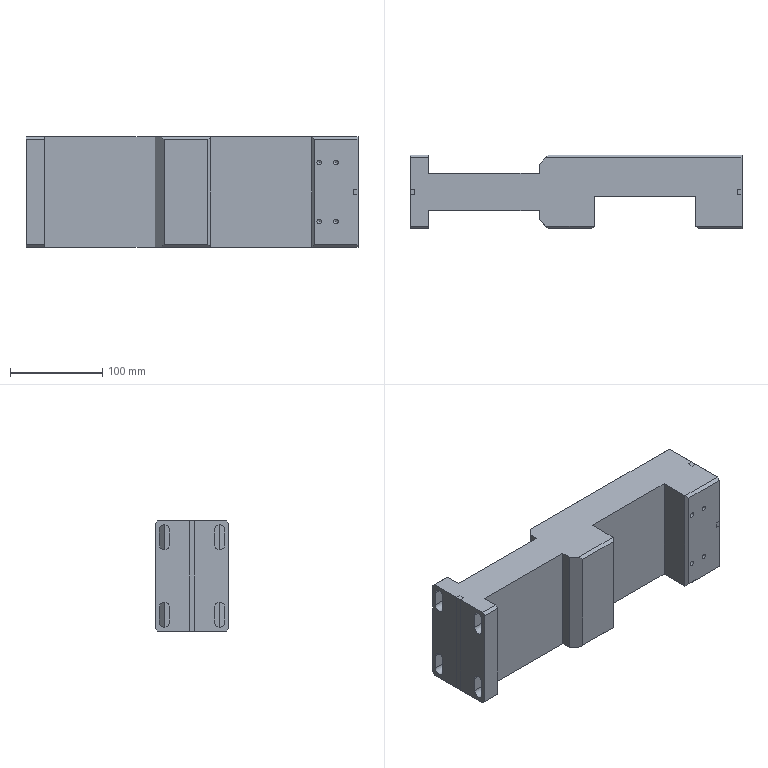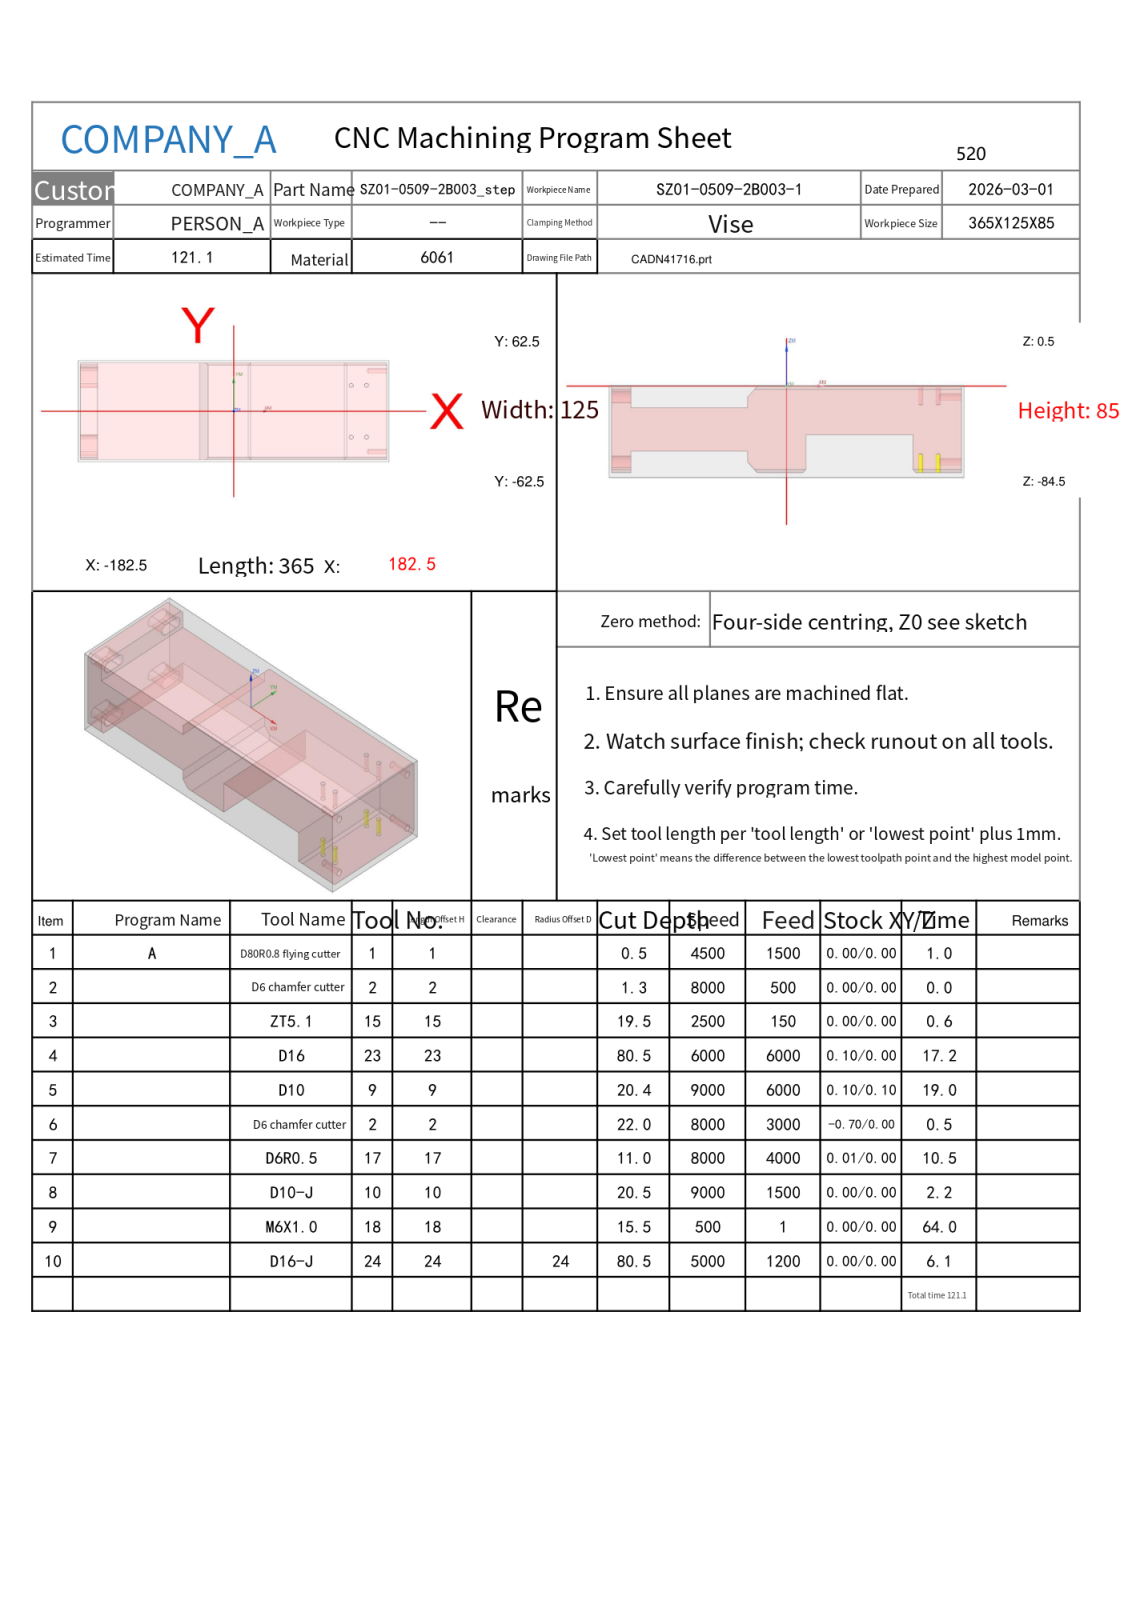NC program | NX | posted by the shop | part box 360 x 80 x 120 mm
Lines 1 to 903 of 6444:
%
O0001
(Machine time: 182.87 MIN)
(===Total Tool:9===)
(T1=D80R0.8 flying cutter D=80.  R=0.8  D-  H01 Z=0.    )
(T2=D6 chamfer cutter   D=6.   R=0.   D-  H02 Z=-21.5 )
(T15=ZT5.1  D=5.1  DR_a=118 D-  H15 Z=-19.  )
(T23=D16    D=16.  R=0.   D-  H23 Z=-80.  )
(T9=D10     D=10.  R=0.   D-  H09 Z=-19.9 )
(T17=D6R0.5 D=6.   R=0.5  D-  H17 Z=-10.5 )
(T10=D10-J  D=10.  R=0.   D10 H10 Z=-20.  )
(T18=M6X1.0 D=5.   DR_a=180 D-  H18 Z=-15.  )
(T24=D16-J  D=16.  R=0.   D24 H24 Z=-80.  )
G80 G90 G17 G49 G40
G91 G28 Z0
M01
N1 T01 M06
(D80R0.8 flying cutter  D=80. R=0.8 H=01 ce=0.00 di=0.00)
G00 G90 G54 X225. Y-50. M03 S4500
G43 H01 Z50.
M08
Z2.
G01 Z0.0 F1500.
X220.
X-220.
Y0.0
X220.
Y50.
X-220.
X-225.
Z2.
G00 Z50.
G91 G28 Z0.0
M05
M09
G91 G28 Z0.0
M01
N2 T02 M06
(D6 chamfer cutter  D=6. R=0. H=02 ce=0.00 di=0.00)
G00 G90 G54 X138. Y-32. M03 S8000
G43 H02 Z50.
M08
G98 G81 X138. Y-32. Z-.8 R1. F500.
X156.
Y32.
X138.
G80
G00 Z50.
G91 G28 Z0.0
M05
M09
G91 G28 Z0.0
M01
N3 T15 M06
(ZT5.1 D=5.1 DR_a=118 H=15)
G00 G90 G54 X138. Y-32. M03 S2500
G43 H15 Z50.
M08
G98 G83 X138. Y-32. Z-19. R1. F150. Q3.
X156.
Y32.
X138.
G80
G00 Z50.
G91 G28 Z0.0
M05
M09
G91 G28 Z0.0
M01
N4 T23 M06
(D16  D=16. R=0. H=23 ce=0.10 di=0.00)
G00 G90 G54 X0.0 Y68.1 M03 S6000
G43 H23 Z50.
M08
Z.5
G01 X180. Z.358 F6000.
G02 X188.1 Y60. Z.348 I0.0 J-8.1
G01 Y-60. Z.253
G02 X180. Y-68.1 Z.243 I-8.1 J0.0
G01 X-180. Z-.04
G02 X-188.1 Y-60. Z-.05 I0.0 J8.1
G01 Y60. Z-.145
G02 X-180. Y68.1 Z-.155 I8.1 J0.0
G01 X180. Z-.439
G02 X188.1 Y60. Z-.449 I0.0 J-8.1
G01 Y-60. Z-.544
G02 X180. Y-68.1 Z-.554 I-8.1 J0.0
G01 X-180. Z-.837
G02 X-188.1 Y-60. Z-.847 I0.0 J8.1
G01 Y60. Z-.942
G02 X-180. Y68.1 Z-.952 I8.1 J0.0
G01 X180. Z-1.236
G02 X188.1 Y60. Z-1.246 I0.0 J-8.1
G01 Y-60. Z-1.341
G02 X180. Y-68.1 Z-1.351 I-8.1 J0.0
G01 X-180. Z-1.634
G02 X-188.1 Y-60. Z-1.645 I0.0 J8.1
G01 Y60. Z-1.739
G02 X-180. Y68.1 Z-1.749 I8.1 J0.0
G01 X180. Z-2.033
G02 X188.1 Y60. Z-2.043 I0.0 J-8.1
G01 Y-60. Z-2.138
G02 X180. Y-68.1 Z-2.148 I-8.1 J0.0
G01 X-180. Z-2.432
G02 X-188.1 Y-60. Z-2.442 I0.0 J8.1
G01 Y60. Z-2.536
G02 X-180. Y68.1 Z-2.546 I8.1 J0.0
G01 X180. Z-2.83
G02 X188.1 Y60. Z-2.84 I0.0 J-8.1
G01 Y-60. Z-2.935
G02 X180. Y-68.1 Z-2.945 I-8.1 J0.0
G01 X-180. Z-3.229
G02 X-188.1 Y-60. Z-3.239 I0.0 J8.1
G01 Y60. Z-3.333
G02 X-180. Y68.1 Z-3.343 I8.1 J0.0
G01 X180. Z-3.627
G02 X188.1 Y60. Z-3.637 I0.0 J-8.1
G01 Y-60. Z-3.732
G02 X180. Y-68.1 Z-3.742 I-8.1 J0.0
G01 X-180. Z-4.026
G02 X-188.1 Y-60. Z-4.036 I0.0 J8.1
G01 Y60. Z-4.13
G02 X-180. Y68.1 Z-4.14 I8.1 J0.0
G01 X180. Z-4.424
G02 X188.1 Y60. Z-4.434 I0.0 J-8.1
G01 Y-60. Z-4.529
G02 X180. Y-68.1 Z-4.539 I-8.1 J0.0
G01 X-180. Z-4.823
G02 X-188.1 Y-60. Z-4.833 I0.0 J8.1
G01 Y60. Z-4.927
G02 X-180. Y68.1 Z-4.937 I8.1 J0.0
G01 X180. Z-5.221
G02 X188.1 Y60. Z-5.231 I0.0 J-8.1
G01 Y-60. Z-5.326
G02 X180. Y-68.1 Z-5.336 I-8.1 J0.0
G01 X-180. Z-5.62
G02 X-188.1 Y-60. Z-5.63 I0.0 J8.1
G01 Y60. Z-5.724
G02 X-180. Y68.1 Z-5.734 I8.1 J0.0
G01 X180. Z-6.018
G02 X188.1 Y60. Z-6.028 I0.0 J-8.1
G01 Y-60. Z-6.123
G02 X180. Y-68.1 Z-6.133 I-8.1 J0.0
G01 X-180. Z-6.417
G02 X-188.1 Y-60. Z-6.427 I0.0 J8.1
G01 Y60. Z-6.521
G02 X-180. Y68.1 Z-6.531 I8.1 J0.0
G01 X180. Z-6.815
G02 X188.1 Y60. Z-6.825 I0.0 J-8.1
G01 Y-60. Z-6.92
G02 X180. Y-68.1 Z-6.93 I-8.1 J0.0
G01 X-180. Z-7.214
G02 X-188.1 Y-60. Z-7.224 I0.0 J8.1
G01 Y60. Z-7.318
G02 X-180. Y68.1 Z-7.328 I8.1 J0.0
G01 X180. Z-7.612
G02 X188.1 Y60. Z-7.622 I0.0 J-8.1
G01 Y-60. Z-7.717
G02 X180. Y-68.1 Z-7.727 I-8.1 J0.0
G01 X-180. Z-8.011
G02 X-188.1 Y-60. Z-8.021 I0.0 J8.1
G01 Y60. Z-8.115
G02 X-180. Y68.1 Z-8.125 I8.1 J0.0
G01 X180. Z-8.409
G02 X188.1 Y60. Z-8.419 I0.0 J-8.1
G01 Y-60. Z-8.514
G02 X180. Y-68.1 Z-8.524 I-8.1 J0.0
G01 X-180. Z-8.808
G02 X-188.1 Y-60. Z-8.818 I0.0 J8.1
G01 Y60. Z-8.912
G02 X-180. Y68.1 Z-8.922 I8.1 J0.0
G01 X180. Z-9.206
G02 X188.1 Y60. Z-9.216 I0.0 J-8.1
G01 Y-60. Z-9.311
G02 X180. Y-68.1 Z-9.321 I-8.1 J0.0
G01 X-180. Z-9.605
G02 X-188.1 Y-60. Z-9.615 I0.0 J8.1
G01 Y60. Z-9.709
G02 X-180. Y68.1 Z-9.719 I8.1 J0.0
G01 X180. Z-10.003
G02 X188.1 Y60. Z-10.013 I0.0 J-8.1
G01 Y-60. Z-10.108
G02 X180. Y-68.1 Z-10.118 I-8.1 J0.0
G01 X-180. Z-10.402
G02 X-188.1 Y-60. Z-10.412 I0.0 J8.1
G01 Y60. Z-10.506
G02 X-180. Y68.1 Z-10.516 I8.1 J0.0
G01 X180. Z-10.8
G02 X188.1 Y60. Z-10.81 I0.0 J-8.1
G01 Y-60. Z-10.905
G02 X180. Y-68.1 Z-10.915 I-8.1 J0.0
G01 X-180. Z-11.199
G02 X-188.1 Y-60. Z-11.209 I0.0 J8.1
G01 Y60. Z-11.303
G02 X-180. Y68.1 Z-11.314 I8.1 J0.0
G01 X180. Z-11.597
G02 X188.1 Y60. Z-11.607 I0.0 J-8.1
G01 Y-60. Z-11.702
G02 X180. Y-68.1 Z-11.712 I-8.1 J0.0
G01 X-180. Z-11.996
G02 X-188.1 Y-60. Z-12.006 I0.0 J8.1
G01 Y60. Z-12.101
G02 X-180. Y68.1 Z-12.111 I8.1 J0.0
G01 X180. Z-12.394
G02 X188.1 Y60. Z-12.404 I0.0 J-8.1
G01 Y-60. Z-12.499
G02 X180. Y-68.1 Z-12.509 I-8.1 J0.0
G01 X-180. Z-12.793
G02 X-188.1 Y-60. Z-12.803 I0.0 J8.1
G01 Y60. Z-12.898
G02 X-180. Y68.1 Z-12.908 I8.1 J0.0
G01 X180. Z-13.191
G02 X188.1 Y60. Z-13.201 I0.0 J-8.1
G01 Y-60. Z-13.296
G02 X180. Y-68.1 Z-13.306 I-8.1 J0.0
G01 X-180. Z-13.59
G02 X-188.1 Y-60. Z-13.6 I0.0 J8.1
G01 Y60. Z-13.695
G02 X-180. Y68.1 Z-13.705 I8.1 J0.0
G01 X180. Z-13.988
G02 X188.1 Y60. Z-13.998 I0.0 J-8.1
G01 Y-60. Z-14.093
G02 X180. Y-68.1 Z-14.103 I-8.1 J0.0
G01 X-180. Z-14.387
G02 X-188.1 Y-60. Z-14.397 I0.0 J8.1
G01 Y60. Z-14.492
G02 X-180. Y68.1 Z-14.502 I8.1 J0.0
G01 X180. Z-14.785
G02 X188.1 Y60. Z-14.796 I0.0 J-8.1
G01 Y-60. Z-14.89
G02 X180. Y-68.1 Z-14.9 I-8.1 J0.0
G01 X-180. Z-15.184
G02 X-188.1 Y-60. Z-15.194 I0.0 J8.1
G01 Y60. Z-15.289
G02 X-180. Y68.1 Z-15.299 I8.1 J0.0
G01 X180. Z-15.583
G02 X188.1 Y60. Z-15.593 I0.0 J-8.1
G01 Y-60. Z-15.687
G02 X180. Y-68.1 Z-15.697 I-8.1 J0.0
G01 X-180. Z-15.981
G02 X-188.1 Y-60. Z-15.991 I0.0 J8.1
G01 Y60. Z-16.086
G02 X-180. Y68.1 Z-16.096 I8.1 J0.0
G01 X180. Z-16.38
G02 X188.1 Y60. Z-16.39 I0.0 J-8.1
G01 Y-60. Z-16.484
G02 X180. Y-68.1 Z-16.494 I-8.1 J0.0
G01 X-180. Z-16.778
G02 X-188.1 Y-60. Z-16.788 I0.0 J8.1
G01 Y60. Z-16.883
G02 X-180. Y68.1 Z-16.893 I8.1 J0.0
G01 X180. Z-17.177
G02 X188.1 Y60. Z-17.187 I0.0 J-8.1
G01 Y-60. Z-17.281
G02 X180. Y-68.1 Z-17.291 I-8.1 J0.0
G01 X-180. Z-17.575
G02 X-188.1 Y-60. Z-17.585 I0.0 J8.1
G01 Y60. Z-17.68
G02 X-180. Y68.1 Z-17.69 I8.1 J0.0
G01 X180. Z-17.974
G02 X188.1 Y60. Z-17.984 I0.0 J-8.1
G01 Y-60. Z-18.078
G02 X180. Y-68.1 Z-18.088 I-8.1 J0.0
G01 X-180. Z-18.372
G02 X-188.1 Y-60. Z-18.382 I0.0 J8.1
G01 Y60. Z-18.477
G02 X-180. Y68.1 Z-18.487 I8.1 J0.0
G01 X180. Z-18.771
G02 X188.1 Y60. Z-18.781 I0.0 J-8.1
G01 Y-60. Z-18.875
G02 X180. Y-68.1 Z-18.885 I-8.1 J0.0
G01 X-180. Z-19.169
G02 X-188.1 Y-60. Z-19.179 I0.0 J8.1
G01 Y60. Z-19.274
G02 X-180. Y68.1 Z-19.284 I8.1 J0.0
G01 X180. Z-19.568
G02 X188.1 Y60. Z-19.578 I0.0 J-8.1
G01 Y-60. Z-19.672
G02 X180. Y-68.1 Z-19.682 I-8.1 J0.0
G01 X-180. Z-19.966
G02 X-188.1 Y-60. Z-19.976 I0.0 J8.1
G01 Y60. Z-20.071
G02 X-180. Y68.1 Z-20.081 I8.1 J0.0
G01 X180. Z-20.365
G02 X188.1 Y60. Z-20.375 I0.0 J-8.1
G01 Y-60. Z-20.469
G02 X180. Y-68.1 Z-20.479 I-8.1 J0.0
G01 X-180. Z-20.763
G02 X-188.1 Y-60. Z-20.773 I0.0 J8.1
G01 Y60. Z-20.868
G02 X-180. Y68.1 Z-20.878 I8.1 J0.0
G01 X180. Z-21.162
G02 X188.1 Y60. Z-21.172 I0.0 J-8.1
G01 Y-60. Z-21.266
G02 X180. Y-68.1 Z-21.276 I-8.1 J0.0
G01 X-180. Z-21.56
G02 X-188.1 Y-60. Z-21.57 I0.0 J8.1
G01 Y60. Z-21.665
G02 X-180. Y68.1 Z-21.675 I8.1 J0.0
G01 X180. Z-21.959
G02 X188.1 Y60. Z-21.969 I0.0 J-8.1
G01 Y-60. Z-22.063
G02 X180. Y-68.1 Z-22.073 I-8.1 J0.0
G01 X-180. Z-22.357
G02 X-188.1 Y-60. Z-22.367 I0.0 J8.1
G01 Y60. Z-22.462
G02 X-180. Y68.1 Z-22.472 I8.1 J0.0
G01 X180. Z-22.756
G02 X188.1 Y60. Z-22.766 I0.0 J-8.1
G01 Y-60. Z-22.86
G02 X180. Y-68.1 Z-22.87 I-8.1 J0.0
G01 X-180. Z-23.154
G02 X-188.1 Y-60. Z-23.164 I0.0 J8.1
G01 Y60. Z-23.259
G02 X-180. Y68.1 Z-23.269 I8.1 J0.0
G01 X180. Z-23.553
G02 X188.1 Y60. Z-23.563 I0.0 J-8.1
G01 Y-60. Z-23.657
G02 X180. Y-68.1 Z-23.667 I-8.1 J0.0
G01 X-180. Z-23.951
G02 X-188.1 Y-60. Z-23.961 I0.0 J8.1
G01 Y60. Z-24.056
G02 X-180. Y68.1 Z-24.066 I8.1 J0.0
G01 X180. Z-24.35
G02 X188.1 Y60. Z-24.36 I0.0 J-8.1
G01 Y-60. Z-24.454
G02 X180. Y-68.1 Z-24.465 I-8.1 J0.0
G01 X-180. Z-24.748
G02 X-188.1 Y-60. Z-24.758 I0.0 J8.1
G01 Y60. Z-24.853
G02 X-180. Y68.1 Z-24.863 I8.1 J0.0
G01 X180. Z-25.147
G02 X188.1 Y60. Z-25.157 I0.0 J-8.1
G01 Y-60. Z-25.252
G02 X180. Y-68.1 Z-25.262 I-8.1 J0.0
G01 X-180. Z-25.545
G02 X-188.1 Y-60. Z-25.555 I0.0 J8.1
G01 Y60. Z-25.65
G02 X-180. Y68.1 Z-25.66 I8.1 J0.0
G01 X180. Z-25.944
G02 X188.1 Y60. Z-25.954 I0.0 J-8.1
G01 Y-60. Z-26.049
G02 X180. Y-68.1 Z-26.059 I-8.1 J0.0
G01 X-180. Z-26.342
G02 X-188.1 Y-60. Z-26.352 I0.0 J8.1
G01 Y60. Z-26.447
G02 X-180. Y68.1 Z-26.457 I8.1 J0.0
G01 X180. Z-26.741
G02 X188.1 Y60. Z-26.751 I0.0 J-8.1
G01 Y-60. Z-26.846
G02 X180. Y-68.1 Z-26.856 I-8.1 J0.0
G01 X-180. Z-27.139
G02 X-188.1 Y-60. Z-27.149 I0.0 J8.1
G01 Y60. Z-27.244
G02 X-180. Y68.1 Z-27.254 I8.1 J0.0
G01 X180. Z-27.538
G02 X188.1 Y60. Z-27.548 I0.0 J-8.1
G01 Y-60. Z-27.643
G02 X180. Y-68.1 Z-27.653 I-8.1 J0.0
G01 X-180. Z-27.936
G02 X-188.1 Y-60. Z-27.947 I0.0 J8.1
G01 Y60. Z-28.041
G02 X-180. Y68.1 Z-28.051 I8.1 J0.0
G01 X180. Z-28.335
G02 X188.1 Y60. Z-28.345 I0.0 J-8.1
G01 Y-60. Z-28.44
G02 X180. Y-68.1 Z-28.45 I-8.1 J0.0
G01 X-180. Z-28.734
G02 X-188.1 Y-60. Z-28.744 I0.0 J8.1
G01 Y60. Z-28.838
G02 X-180. Y68.1 Z-28.848 I8.1 J0.0
G01 X180. Z-29.132
G02 X188.1 Y60. Z-29.142 I0.0 J-8.1
G01 Y-60. Z-29.237
G02 X180. Y-68.1 Z-29.247 I-8.1 J0.0
G01 X-180. Z-29.531
G02 X-188.1 Y-60. Z-29.541 I0.0 J8.1
G01 Y60. Z-29.635
G02 X-180. Y68.1 Z-29.645 I8.1 J0.0
G01 X180. Z-29.929
G02 X188.1 Y60. Z-29.939 I0.0 J-8.1
G01 Y-60. Z-30.034
G02 X180. Y-68.1 Z-30.044 I-8.1 J0.0
G01 X-180. Z-30.328
G02 X-188.1 Y-60. Z-30.338 I0.0 J8.1
G01 Y60. Z-30.432
G02 X-180. Y68.1 Z-30.442 I8.1 J0.0
G01 X180. Z-30.726
G02 X188.1 Y60. Z-30.736 I0.0 J-8.1
G01 Y-60. Z-30.831
G02 X180. Y-68.1 Z-30.841 I-8.1 J0.0
G01 X-180. Z-31.125
G02 X-188.1 Y-60. Z-31.135 I0.0 J8.1
G01 Y60. Z-31.229
G02 X-180. Y68.1 Z-31.239 I8.1 J0.0
G01 X180. Z-31.523
G02 X188.1 Y60. Z-31.533 I0.0 J-8.1
G01 Y-60. Z-31.628
G02 X180. Y-68.1 Z-31.638 I-8.1 J0.0
G01 X-180. Z-31.922
G02 X-188.1 Y-60. Z-31.932 I0.0 J8.1
G01 Y60. Z-32.026
G02 X-180. Y68.1 Z-32.036 I8.1 J0.0
G01 X180. Z-32.32
G02 X188.1 Y60. Z-32.33 I0.0 J-8.1
G01 Y-60. Z-32.425
G02 X180. Y-68.1 Z-32.435 I-8.1 J0.0
G01 X-180. Z-32.719
G02 X-188.1 Y-60. Z-32.729 I0.0 J8.1
G01 Y60. Z-32.823
G02 X-180. Y68.1 Z-32.833 I8.1 J0.0
G01 X180. Z-33.117
G02 X188.1 Y60. Z-33.127 I0.0 J-8.1
G01 Y-60. Z-33.222
G02 X180. Y-68.1 Z-33.232 I-8.1 J0.0
G01 X-180. Z-33.516
G02 X-188.1 Y-60. Z-33.526 I0.0 J8.1
G01 Y60. Z-33.62
G02 X-180. Y68.1 Z-33.63 I8.1 J0.0
G01 X180. Z-33.914
G02 X188.1 Y60. Z-33.924 I0.0 J-8.1
G01 Y-60. Z-34.019
G02 X180. Y-68.1 Z-34.029 I-8.1 J0.0
G01 X-180. Z-34.313
G02 X-188.1 Y-60. Z-34.323 I0.0 J8.1
G01 Y60. Z-34.417
G02 X-180. Y68.1 Z-34.427 I8.1 J0.0
G01 X180. Z-34.711
G02 X188.1 Y60. Z-34.721 I0.0 J-8.1
G01 Y-60. Z-34.816
G02 X180. Y-68.1 Z-34.826 I-8.1 J0.0
G01 X-180. Z-35.11
G02 X-188.1 Y-60. Z-35.12 I0.0 J8.1
G01 Y60. Z-35.214
G02 X-180. Y68.1 Z-35.224 I8.1 J0.0
G01 X180. Z-35.508
G02 X188.1 Y60. Z-35.518 I0.0 J-8.1
G01 Y-60. Z-35.613
G02 X180. Y-68.1 Z-35.623 I-8.1 J0.0
G01 X-180. Z-35.907
G02 X-188.1 Y-60. Z-35.917 I0.0 J8.1
G01 Y60. Z-36.011
G02 X-180. Y68.1 Z-36.021 I8.1 J0.0
G01 X180. Z-36.305
G02 X188.1 Y60. Z-36.315 I0.0 J-8.1
G01 Y-60. Z-36.41
G02 X180. Y-68.1 Z-36.42 I-8.1 J0.0
G01 X-180. Z-36.704
G02 X-188.1 Y-60. Z-36.714 I0.0 J8.1
G01 Y60. Z-36.808
G02 X-180. Y68.1 Z-36.818 I8.1 J0.0
G01 X180. Z-37.102
G02 X188.1 Y60. Z-37.112 I0.0 J-8.1
G01 Y-60. Z-37.207
G02 X180. Y-68.1 Z-37.217 I-8.1 J0.0
G01 X-180. Z-37.501
G02 X-188.1 Y-60. Z-37.511 I0.0 J8.1
G01 Y60. Z-37.605
G02 X-180. Y68.1 Z-37.616 I8.1 J0.0
G01 X180. Z-37.899
G02 X188.1 Y60. Z-37.909 I0.0 J-8.1
G01 Y-60. Z-38.004
G02 X180. Y-68.1 Z-38.014 I-8.1 J0.0
G01 X-180. Z-38.298
G02 X-188.1 Y-60. Z-38.308 I0.0 J8.1
G01 Y60. Z-38.403
G02 X-180. Y68.1 Z-38.413 I8.1 J0.0
G01 X180. Z-38.696
G02 X188.1 Y60. Z-38.706 I0.0 J-8.1
G01 Y-60. Z-38.801
G02 X180. Y-68.1 Z-38.811 I-8.1 J0.0
G01 X-180. Z-39.095
G02 X-188.1 Y-60. Z-39.105 I0.0 J8.1
G01 Y60. Z-39.2
G02 X-180. Y68.1 Z-39.21 I8.1 J0.0
G01 X180. Z-39.493
G02 X188.1 Y60. Z-39.503 I0.0 J-8.1
G01 Y-60. Z-39.598
G02 X180. Y-68.1 Z-39.608 I-8.1 J0.0
G01 X-180. Z-39.892
G02 X-188.1 Y-60. Z-39.902 I0.0 J8.1
G01 Y60. Z-39.997
G02 X-180. Y68.1 Z-40.007 I8.1 J0.0
G01 X180. Z-40.29
G02 X188.1 Y60. Z-40.3 I0.0 J-8.1
G01 Y-60. Z-40.395
G02 X180. Y-68.1 Z-40.405 I-8.1 J0.0
G01 X-180. Z-40.689
G02 X-188.1 Y-60. Z-40.699 I0.0 J8.1
G01 Y60. Z-40.794
G02 X-180. Y68.1 Z-40.804 I8.1 J0.0
G01 X180. Z-41.087
G02 X188.1 Y60. Z-41.097 I0.0 J-8.1
G01 Y-60. Z-41.192
G02 X180. Y-68.1 Z-41.202 I-8.1 J0.0
G01 X-180. Z-41.486
G02 X-188.1 Y-60. Z-41.496 I0.0 J8.1
G01 Y60. Z-41.591
G02 X-180. Y68.1 Z-41.601 I8.1 J0.0
G01 X180. Z-41.884
G02 X188.1 Y60. Z-41.895 I0.0 J-8.1
G01 Y-60. Z-41.989
G02 X180. Y-68.1 Z-41.999 I-8.1 J0.0
G01 X-180. Z-42.283
G02 X-188.1 Y-60. Z-42.293 I0.0 J8.1
G01 Y60. Z-42.388
G02 X-180. Y68.1 Z-42.398 I8.1 J0.0
G01 X180. Z-42.682
G02 X188.1 Y60. Z-42.692 I0.0 J-8.1
G01 Y-60. Z-42.786
G02 X180. Y-68.1 Z-42.796 I-8.1 J0.0
G01 X-180. Z-43.08
G02 X-188.1 Y-60. Z-43.09 I0.0 J8.1
G01 Y60. Z-43.185
G02 X-180. Y68.1 Z-43.195 I8.1 J0.0
G01 X180. Z-43.479
G02 X188.1 Y60. Z-43.489 I0.0 J-8.1
G01 Y-60. Z-43.583
G02 X180. Y-68.1 Z-43.593 I-8.1 J0.0
G01 X-180. Z-43.877
G02 X-188.1 Y-60. Z-43.887 I0.0 J8.1
G01 Y60. Z-43.982
G02 X-180. Y68.1 Z-43.992 I8.1 J0.0
G01 X180. Z-44.276
G02 X188.1 Y60. Z-44.286 I0.0 J-8.1
G01 Y-60. Z-44.38
G02 X180. Y-68.1 Z-44.39 I-8.1 J0.0
G01 X-180. Z-44.674
G02 X-188.1 Y-60. Z-44.684 I0.0 J8.1
G01 Y60. Z-44.779
G02 X-180. Y68.1 Z-44.789 I8.1 J0.0
G01 X180. Z-45.073
G02 X188.1 Y60. Z-45.083 I0.0 J-8.1
G01 Y-60. Z-45.177
G02 X180. Y-68.1 Z-45.187 I-8.1 J0.0
G01 X-180. Z-45.471
G02 X-188.1 Y-60. Z-45.481 I0.0 J8.1
G01 Y60. Z-45.576
G02 X-180. Y68.1 Z-45.586 I8.1 J0.0
G01 X180. Z-45.87
G02 X188.1 Y60. Z-45.88 I0.0 J-8.1
G01 Y-60. Z-45.974
G02 X180. Y-68.1 Z-45.984 I-8.1 J0.0
G01 X-180. Z-46.268
G02 X-188.1 Y-60. Z-46.278 I0.0 J8.1
G01 Y60. Z-46.373
G02 X-180. Y68.1 Z-46.383 I8.1 J0.0
G01 X180. Z-46.667
G02 X188.1 Y60. Z-46.677 I0.0 J-8.1
G01 Y-60. Z-46.771
G02 X180. Y-68.1 Z-46.781 I-8.1 J0.0
G01 X-180. Z-47.065
G02 X-188.1 Y-60. Z-47.075 I0.0 J8.1
G01 Y60. Z-47.17
G02 X-180. Y68.1 Z-47.18 I8.1 J0.0
G01 X180. Z-47.464
G02 X188.1 Y60. Z-47.474 I0.0 J-8.1
G01 Y-60. Z-47.568
G02 X180. Y-68.1 Z-47.578 I-8.1 J0.0
G01 X-180. Z-47.862
G02 X-188.1 Y-60. Z-47.872 I0.0 J8.1
G01 Y60. Z-47.967
G02 X-180. Y68.1 Z-47.977 I8.1 J0.0
G01 X180. Z-48.261
G02 X188.1 Y60. Z-48.271 I0.0 J-8.1
G01 Y-60. Z-48.365
G02 X180. Y-68.1 Z-48.375 I-8.1 J0.0
G01 X-180. Z-48.659
G02 X-188.1 Y-60. Z-48.669 I0.0 J8.1
G01 Y60. Z-48.764
G02 X-180. Y68.1 Z-48.774 I8.1 J0.0
G01 X180. Z-49.058
G02 X188.1 Y60. Z-49.068 I0.0 J-8.1
G01 Y-60. Z-49.162
G02 X180. Y-68.1 Z-49.172 I-8.1 J0.0
G01 X-180. Z-49.456
G02 X-188.1 Y-60. Z-49.466 I0.0 J8.1
G01 Y60. Z-49.561
G02 X-180. Y68.1 Z-49.571 I8.1 J0.0
G01 X180. Z-49.855
G02 X188.1 Y60. Z-49.865 I0.0 J-8.1
G01 Y-60. Z-49.959
G02 X180. Y-68.1 Z-49.969 I-8.1 J0.0
G01 X-180. Z-50.253
G02 X-188.1 Y-60. Z-50.263 I0.0 J8.1
G01 Y60. Z-50.358
G02 X-180. Y68.1 Z-50.368 I8.1 J0.0
G01 X180. Z-50.652
G02 X188.1 Y60. Z-50.662 I0.0 J-8.1
G01 Y-60. Z-50.756
G02 X180. Y-68.1 Z-50.766 I-8.1 J0.0
G01 X-180. Z-51.05
G02 X-188.1 Y-60. Z-51.06 I0.0 J8.1
G01 Y60. Z-51.155
G02 X-180. Y68.1 Z-51.165 I8.1 J0.0
G01 X180. Z-51.449
G02 X188.1 Y60. Z-51.459 I0.0 J-8.1
G01 Y-60. Z-51.553
G02 X180. Y-68.1 Z-51.564 I-8.1 J0.0
G01 X-180. Z-51.847
G02 X-188.1 Y-60. Z-51.857 I0.0 J8.1
G01 Y60. Z-51.952
G02 X-180. Y68.1 Z-51.962 I8.1 J0.0
G01 X180. Z-52.246
G02 X188.1 Y60. Z-52.256 I0.0 J-8.1
G01 Y-60. Z-52.351
G02 X180. Y-68.1 Z-52.361 I-8.1 J0.0
G01 X-180. Z-52.644
G02 X-188.1 Y-60. Z-52.654 I0.0 J8.1
G01 Y60. Z-52.749
G02 X-180. Y68.1 Z-52.759 I8.1 J0.0
G01 X180. Z-53.043
G02 X188.1 Y60. Z-53.053 I0.0 J-8.1
G01 Y-60. Z-53.148
G02 X180. Y-68.1 Z-53.158 I-8.1 J0.0
G01 X-180. Z-53.441
G02 X-188.1 Y-60. Z-53.451 I0.0 J8.1
G01 Y60. Z-53.546
G02 X-180. Y68.1 Z-53.556 I8.1 J0.0
G01 X180. Z-53.84
G02 X188.1 Y60. Z-53.85 I0.0 J-8.1
G01 Y-60. Z-53.945
G02 X180. Y-68.1 Z-53.955 I-8.1 J0.0
G01 X-180. Z-54.238
G02 X-188.1 Y-60. Z-54.248 I0.0 J8.1
G01 Y60. Z-54.343
G02 X-180. Y68.1 Z-54.353 I8.1 J0.0
G01 X180. Z-54.637
G02 X188.1 Y60. Z-54.647 I0.0 J-8.1
G01 Y-60. Z-54.742
G02 X180. Y-68.1 Z-54.752 I-8.1 J0.0
G01 X-180. Z-55.035
G02 X-188.1 Y-60. Z-55.046 I0.0 J8.1
G01 Y60. Z-55.14
G02 X-180. Y68.1 Z-55.15 I8.1 J0.0
G01 X180. Z-55.434
G02 X188.1 Y60. Z-55.444 I0.0 J-8.1
G01 Y-60. Z-55.539
G02 X180. Y-68.1 Z-55.549 I-8.1 J0.0
G01 X-180. Z-55.833
G02 X-188.1 Y-60. Z-55.843 I0.0 J8.1
G01 Y60. Z-55.937
G02 X-180. Y68.1 Z-55.947 I8.1 J0.0
G01 X180. Z-56.231
G02 X188.1 Y60. Z-56.241 I0.0 J-8.1
G01 Y-60. Z-56.336
G02 X180. Y-68.1 Z-56.346 I-8.1 J0.0
G01 X-180. Z-56.63
G02 X-188.1 Y-60. Z-56.64 I0.0 J8.1
G01 Y60. Z-56.734
G02 X-180. Y68.1 Z-56.744 I8.1 J0.0
G01 X180. Z-57.028
G02 X188.1 Y60. Z-57.038 I0.0 J-8.1
G01 Y-60. Z-57.133
G02 X180. Y-68.1 Z-57.143 I-8.1 J0.0
G01 X-180. Z-57.427
G02 X-188.1 Y-60. Z-57.437 I0.0 J8.1
G01 Y60. Z-57.531
G02 X-180. Y68.1 Z-57.541 I8.1 J0.0
G01 X180. Z-57.825
G02 X188.1 Y60. Z-57.835 I0.0 J-8.1
G01 Y-60. Z-57.93
G02 X180. Y-68.1 Z-57.94 I-8.1 J0.0
G01 X-180. Z-58.224
G02 X-188.1 Y-60. Z-58.234 I0.0 J8.1
G01 Y60. Z-58.328
G02 X-180. Y68.1 Z-58.338 I8.1 J0.0
G01 X180. Z-58.622
G02 X188.1 Y60. Z-58.632 I0.0 J-8.1
G01 Y-60. Z-58.727
G02 X180. Y-68.1 Z-58.737 I-8.1 J0.0
G01 X-180. Z-59.021
G02 X-188.1 Y-60. Z-59.031 I0.0 J8.1
G01 Y60. Z-59.125
G02 X-180. Y68.1 Z-59.135 I8.1 J0.0
G01 X180. Z-59.419
G02 X188.1 Y60. Z-59.429 I0.0 J-8.1
G01 Y-60. Z-59.524
G02 X180. Y-68.1 Z-59.534 I-8.1 J0.0
G01 X-180. Z-59.818
G02 X-188.1 Y-60. Z-59.828 I0.0 J8.1
G01 Y60. Z-59.922
G02 X-180. Y68.1 Z-59.932 I8.1 J0.0
G01 X180. Z-60.216
G02 X188.1 Y60. Z-60.226 I0.0 J-8.1
G01 Y-60. Z-60.321
G02 X180. Y-68.1 Z-60.331 I-8.1 J0.0
G01 X-180. Z-60.615
G02 X-188.1 Y-60. Z-60.625 I0.0 J8.1
G01 Y60. Z-60.719
G02 X-180. Y68.1 Z-60.729 I8.1 J0.0
G01 X180. Z-61.013
G02 X188.1 Y60. Z-61.023 I0.0 J-8.1
G01 Y-60. Z-61.118
G02 X180. Y-68.1 Z-61.128 I-8.1 J0.0
G01 X-180. Z-61.412
G02 X-188.1 Y-60. Z-61.422 I0.0 J8.1
G01 Y60. Z-61.516
G02 X-180. Y68.1 Z-61.526 I8.1 J0.0
G01 X180. Z-61.81
G02 X188.1 Y60. Z-61.82 I0.0 J-8.1
G01 Y-60. Z-61.915
G02 X180. Y-68.1 Z-61.925 I-8.1 J0.0
G01 X-180. Z-62.209
G02 X-188.1 Y-60. Z-62.219 I0.0 J8.1
G01 Y60. Z-62.313
G02 X-180. Y68.1 Z-62.323 I8.1 J0.0
G01 X180. Z-62.607
G02 X188.1 Y60. Z-62.617 I0.0 J-8.1
G01 Y-60. Z-62.712
G02 X180. Y-68.1 Z-62.722 I-8.1 J0.0
G01 X-180. Z-63.006
G02 X-188.1 Y-60. Z-63.016 I0.0 J8.1
G01 Y60. Z-63.11
G02 X-180. Y68.1 Z-63.12 I8.1 J0.0
G01 X180. Z-63.404
G02 X188.1 Y60. Z-63.414 I0.0 J-8.1
G01 Y-60. Z-63.509
G02 X180. Y-68.1 Z-63.519 I-8.1 J0.0
G01 X-180. Z-63.803
G02 X-188.1 Y-60. Z-63.813 I0.0 J8.1
G01 Y60. Z-63.907
G02 X-180. Y68.1 Z-63.917 I8.1 J0.0
G01 X180. Z-64.201
G02 X188.1 Y60. Z-64.211 I0.0 J-8.1
G01 Y-60. Z-64.306
G02 X180. Y-68.1 Z-64.316 I-8.1 J0.0
G01 X-180. Z-64.6
G02 X-188.1 Y-60. Z-64.61 I0.0 J8.1
G01 Y60. Z-64.704
G02 X-180. Y68.1 Z-64.715 I8.1 J0.0
G01 X180. Z-64.998
G02 X188.1 Y60. Z-65.008 I0.0 J-8.1
G01 Y-60. Z-65.103
G02 X180. Y-68.1 Z-65.113 I-8.1 J0.0
G01 X-180. Z-65.397
G02 X-188.1 Y-60. Z-65.407 I0.0 J8.1
G01 Y60. Z-65.502
G02 X-180. Y68.1 Z-65.512 I8.1 J0.0
G01 X180. Z-65.795
G02 X188.1 Y60. Z-65.805 I0.0 J-8.1
G01 Y-60. Z-65.9
G02 X180. Y-68.1 Z-65.91 I-8.1 J0.0
G01 X-180. Z-66.194
G02 X-188.1 Y-60. Z-66.204 I0.0 J8.1
G01 Y60. Z-66.299
G02 X-180. Y68.1 Z-66.309 I8.1 J0.0
G01 X180. Z-66.592
G02 X188.1 Y60. Z-66.602 I0.0 J-8.1
G01 Y-60. Z-66.697
G02 X180. Y-68.1 Z-66.707 I-8.1 J0.0
G01 X-180. Z-66.991
G02 X-188.1 Y-60. Z-67.001 I0.0 J8.1
G01 Y60. Z-67.096
G02 X-180. Y68.1 Z-67.106 I8.1 J0.0
G01 X180. Z-67.389
G02 X188.1 Y60. Z-67.399 I0.0 J-8.1
G01 Y-60. Z-67.494
G02 X180. Y-68.1 Z-67.504 I-8.1 J0.0
G01 X-180. Z-67.788
G02 X-188.1 Y-60. Z-67.798 I0.0 J8.1
G01 Y60. Z-67.893
G02 X-180. Y68.1 Z-67.903 I8.1 J0.0
G01 X180. Z-68.186
G02 X188.1 Y60. Z-68.197 I0.0 J-8.1
G01 Y-60. Z-68.291
G02 X180. Y-68.1 Z-68.301 I-8.1 J0.0
G01 X-180. Z-68.585
G02 X-188.1 Y-60. Z-68.595 I0.0 J8.1
G01 Y60. Z-68.69
G02 X-180. Y68.1 Z-68.7 I8.1 J0.0
G01 X180. Z-68.984
G02 X188.1 Y60. Z-68.994 I0.0 J-8.1
G01 Y-60. Z-69.088
G02 X180. Y-68.1 Z-69.098 I-8.1 J0.0
G01 X-180. Z-69.382
G02 X-188.1 Y-60. Z-69.392 I0.0 J8.1
G01 Y60. Z-69.487
G02 X-180. Y68.1 Z-69.497 I8.1 J0.0
G01 X180. Z-69.781
G02 X188.1 Y60. Z-69.791 I0.0 J-8.1
G01 Y-60. Z-69.885
G02 X180. Y-68.1 Z-69.895 I-8.1 J0.0
G01 X-180. Z-70.179
G02 X-188.1 Y-60. Z-70.189 I0.0 J8.1
G01 Y60. Z-70.284
G02 X-180. Y68.1 Z-70.294 I8.1 J0.0
G01 X180. Z-70.578
G02 X188.1 Y60. Z-70.588 I0.0 J-8.1
G01 Y-60. Z-70.682
G02 X180. Y-68.1 Z-70.692 I-8.1 J0.0
G01 X-180. Z-70.976
G02 X-188.1 Y-60. Z-70.986 I0.0 J8.1
G01 Y60. Z-71.081
G02 X-180. Y68.1 Z-71.091 I8.1 J0.0
G01 X180. Z-71.375
G02 X188.1 Y60. Z-71.385 I0.0 J-8.1
G01 Y-60. Z-71.479
G02 X180. Y-68.1 Z-71.489 I-8.1 J0.0
G01 X-180. Z-71.773
G02 X-188.1 Y-60. Z-71.783 I0.0 J8.1
G01 Y60. Z-71.878
G02 X-180. Y68.1 Z-71.888 I8.1 J0.0
G01 X180. Z-72.172
G02 X188.1 Y60. Z-72.182 I0.0 J-8.1
G01 Y-60. Z-72.276
G02 X180. Y-68.1 Z-72.286 I-8.1 J0.0
G01 X-180. Z-72.57
G02 X-188.1 Y-60. Z-72.58 I0.0 J8.1
G01 Y60. Z-72.675
G02 X-180. Y68.1 Z-72.685 I8.1 J0.0
G01 X180. Z-72.969
G02 X188.1 Y60. Z-72.979 I0.0 J-8.1
G01 Y-60. Z-73.073
G02 X180. Y-68.1 Z-73.083 I-8.1 J0.0
G01 X-180. Z-73.367
G02 X-188.1 Y-60. Z-73.377 I0.0 J8.1
G01 Y60. Z-73.472
G02 X-180. Y68.1 Z-73.482 I8.1 J0.0
G01 X180. Z-73.766
G02 X188.1 Y60. Z-73.776 I0.0 J-8.1
G01 Y-60. Z-73.87
G02 X180. Y-68.1 Z-73.88 I-8.1 J0.0
G01 X-180. Z-74.164
G02 X-188.1 Y-60. Z-74.174 I0.0 J8.1
G01 Y60. Z-74.269
G02 X-180. Y68.1 Z-74.279 I8.1 J0.0
G01 X180. Z-74.563
G02 X188.1 Y60. Z-74.573 I0.0 J-8.1
G01 Y-60. Z-74.667
G02 X180. Y-68.1 Z-74.677 I-8.1 J0.0
G01 X-180. Z-74.961
G02 X-188.1 Y-60. Z-74.971 I0.0 J8.1
G01 Y60. Z-75.066
G02 X-180. Y68.1 Z-75.076 I8.1 J0.0
G01 X180. Z-75.36
G02 X188.1 Y60. Z-75.37 I0.0 J-8.1
G01 Y-60. Z-75.464
G02 X180. Y-68.1 Z-75.474 I-8.1 J0.0
G01 X-180. Z-75.758
G02 X-188.1 Y-60. Z-75.768 I0.0 J8.1
G01 Y60. Z-75.863
G02 X-180. Y68.1 Z-75.873 I8.1 J0.0
G01 X180. Z-76.157
G02 X188.1 Y60. Z-76.167 I0.0 J-8.1
G01 Y-60. Z-76.261
G02 X180. Y-68.1 Z-76.271 I-8.1 J0.0
G01 X-180. Z-76.555
G02 X-188.1 Y-60. Z-76.565 I0.0 J8.1
G01 Y60. Z-76.66
G02 X-180. Y68.1 Z-76.67 I8.1 J0.0
G01 X180. Z-76.954
G02 X188.1 Y60. Z-76.964 I0.0 J-8.1
G01 Y-60. Z-77.058
G02 X180. Y-68.1 Z-77.068 I-8.1 J0.0
G01 X-180. Z-77.352
G02 X-188.1 Y-60. Z-77.362 I0.0 J8.1
G01 Y60. Z-77.457
G02 X-180. Y68.1 Z-77.467 I8.1 J0.0
G01 X180. Z-77.751
G02 X188.1 Y60. Z-77.761 I0.0 J-8.1
G01 Y-60. Z-77.855
G02 X180. Y-68.1 Z-77.866 I-8.1 J0.0
G01 X-180. Z-78.149
G02 X-188.1 Y-60. Z-78.159 I0.0 J8.1
G01 Y60. Z-78.254
G02 X-180. Y68.1 Z-78.264 I8.1 J0.0
G01 X180. Z-78.548
G02 X188.1 Y60. Z-78.558 I0.0 J-8.1
G01 Y-60. Z-78.653
G02 X180. Y-68.1 Z-78.663 I-8.1 J0.0
G01 X-180. Z-78.946
G02 X-188.1 Y-60. Z-78.956 I0.0 J8.1
G01 Y60. Z-79.051
G02 X-180. Y68.1 Z-79.061 I8.1 J0.0
G01 X180. Z-79.345
G02 X188.1 Y60. Z-79.355 I0.0 J-8.1
G01 Y-60. Z-79.45
G02 X180. Y-68.1 Z-79.46 I-8.1 J0.0
G01 X-180. Z-79.743
G02 X-188.1 Y-60. Z-79.753 I0.0 J8.1
G01 Y60. Z-79.848
G02 X-180. Y68.1 Z-79.858 I8.1 J0.0
G01 X0.0 Z-80.
X180.
G02 X188.1 Y60. I0.0 J-8.1
G01 Y-60.
G02 X180. Y-68.1 I-8.1 J0.0
G01 X-180.
G02 X-188.1 Y-60. I0.0 J8.1
G01 Y60.
G02 X-180. Y68.1 I8.1 J0.0
G01 X0.0
X.5
Z-79.
G00 Z50.
G91 G28 Z0.0
M05
M09
G91 G28 Z0.0
M01